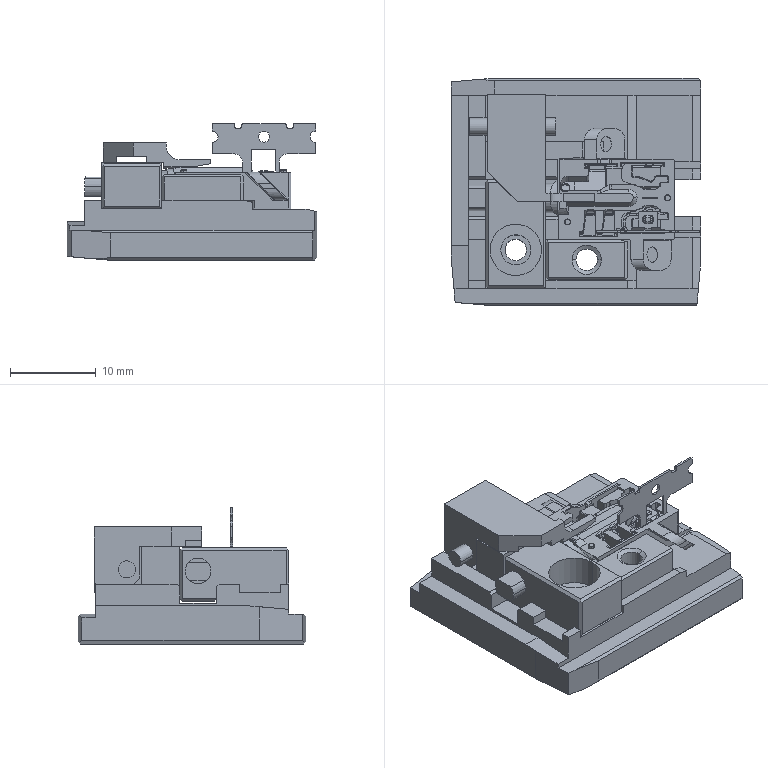Part | NX | 9 solids | 965 faces | box 29 x 26.5 x 15.878 mm | volume 4914 mm3 | plane 532 | cylinder 287 | torus 50 | sphere 48 | cone 28 | spline 20 | commonest cylinder face diameters 0.2 x104 0.4 x17 0.3 x16 1 x15 2 x14 0.7 x13